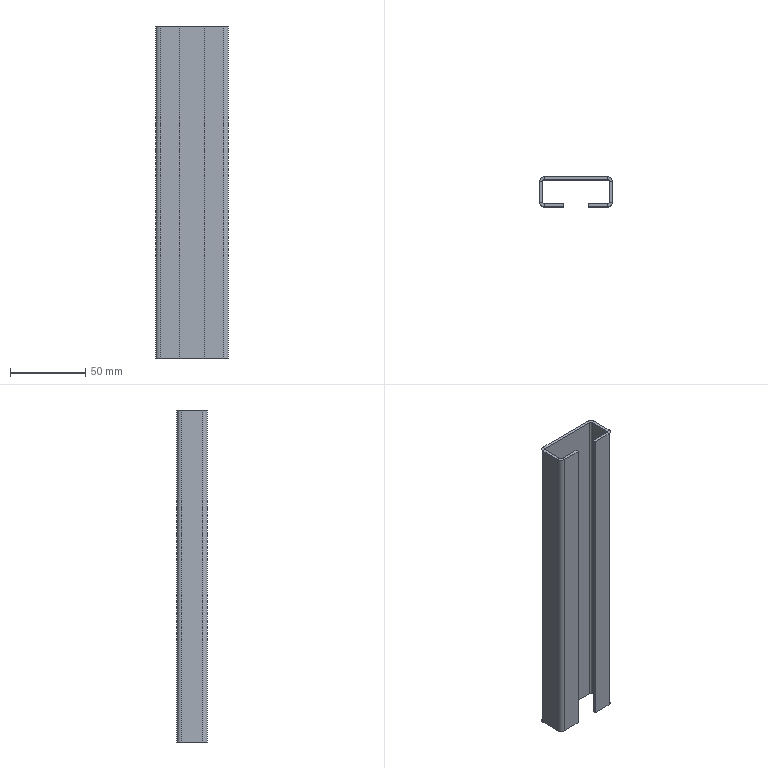Part | 1 solid | 38 faces | box 48 x 20 x 220 mm | volume 47769 mm3 | plane 30 | cylinder 8 | commonest cylinder face diameters 2 x4 6 x4
STEP:
#1=CARTESIAN_POINT('',(-24.,-17.,110.));
#2=VERTEX_POINT('',#1);
#3=CARTESIAN_POINT('',(-22.,-17.,110.));
#4=VERTEX_POINT('',#3);
#5=CARTESIAN_POINT('',(-24.,-17.,110.));
#6=DIRECTION('',(1.,0.,0.));
#7=VECTOR('',#6,1000.);
#8=LINE('',#5,#7);
#9=EDGE_CURVE('',#2,#4,#8,.T.);
#10=ORIENTED_EDGE('',*,*,#9,.F.);
#11=CARTESIAN_POINT('',(-21.,-20.,110.));
#12=VERTEX_POINT('',#11);
#13=CARTESIAN_POINT('',(-21.,-17.,110.));
#14=DIRECTION('',(0.,0.,-1.));
#15=DIRECTION('',(1.,0.,0.));
#16=AXIS2_PLACEMENT_3D('',#13,#14,#15);
#17=CIRCLE('',#16,3.);
#18=EDGE_CURVE('',#12,#2,#17,.T.);
#19=ORIENTED_EDGE('',*,*,#18,.F.);
#20=CARTESIAN_POINT('',(-21.,-18.,110.));
#21=VERTEX_POINT('',#20);
#22=CARTESIAN_POINT('',(-21.,-18.,110.));
#23=DIRECTION('',(0.,-1.,0.));
#24=VECTOR('',#23,1000.);
#25=LINE('',#22,#24);
#26=EDGE_CURVE('',#21,#12,#25,.T.);
#27=ORIENTED_EDGE('',*,*,#26,.F.);
#28=CARTESIAN_POINT('',(-21.,-17.,110.));
#29=DIRECTION('',(0.,0.,-1.));
#30=DIRECTION('',(1.,0.,0.));
#31=AXIS2_PLACEMENT_3D('',#28,#29,#30);
#32=CIRCLE('',#31,1.);
#33=EDGE_CURVE('',#21,#4,#32,.T.);
#34=ORIENTED_EDGE('',*,*,#33,.T.);
#35=EDGE_LOOP('',(#10,#19,#27,#34));
#36=FACE_OUTER_BOUND('',#35,.T.);
#37=CARTESIAN_POINT('',(-24.,-17.,110.));
#38=DIRECTION('',(0.,0.,1.));
#39=DIRECTION('',(1.,0.,0.));
#40=AXIS2_PLACEMENT_3D('',#37,#38,#39);
#41=PLANE('',#40);
#42=ADVANCED_FACE('',(#36),#41,.T.);
#43=CARTESIAN_POINT('',(-24.,-3.,110.));
#44=VERTEX_POINT('',#43);
#45=CARTESIAN_POINT('',(-24.,-20.,110.));
#46=DIRECTION('',(0.,1.,0.));
#47=VECTOR('',#46,1000.);
#48=LINE('',#45,#47);
#49=EDGE_CURVE('',#2,#44,#48,.T.);
#50=ORIENTED_EDGE('',*,*,#49,.F.);
#51=ORIENTED_EDGE('',*,*,#9,.T.);
#52=CARTESIAN_POINT('',(-22.,-3.,110.));
#53=VERTEX_POINT('',#52);
#54=CARTESIAN_POINT('',(-22.,-20.,110.));
#55=DIRECTION('',(0.,1.,0.));
#56=VECTOR('',#55,1000.);
#57=LINE('',#54,#56);
#58=EDGE_CURVE('',#4,#53,#57,.T.);
#59=ORIENTED_EDGE('',*,*,#58,.T.);
#60=CARTESIAN_POINT('',(-22.,-3.,110.));
#61=DIRECTION('',(-1.,0.,0.));
#62=VECTOR('',#61,1000.);
#63=LINE('',#60,#62);
#64=EDGE_CURVE('',#53,#44,#63,.T.);
#65=ORIENTED_EDGE('',*,*,#64,.T.);
#66=EDGE_LOOP('',(#50,#51,#59,#65));
#67=FACE_OUTER_BOUND('',#66,.T.);
#68=CARTESIAN_POINT('',(-21.,-18.,110.));
#69=DIRECTION('',(0.,0.,1.));
#70=DIRECTION('',(1.,0.,0.));
#71=AXIS2_PLACEMENT_3D('',#68,#69,#70);
#72=PLANE('',#71);
#73=ADVANCED_FACE('',(#67),#72,.T.);
#74=CARTESIAN_POINT('',(-21.,-20.,-110.));
#75=VERTEX_POINT('',#74);
#76=CARTESIAN_POINT('',(-21.,-18.,-110.));
#77=VERTEX_POINT('',#76);
#78=CARTESIAN_POINT('',(-21.,-20.,-110.));
#79=DIRECTION('',(0.,1.,0.));
#80=VECTOR('',#79,1000.);
#81=LINE('',#78,#80);
#82=EDGE_CURVE('',#75,#77,#81,.T.);
#83=ORIENTED_EDGE('',*,*,#82,.F.);
#84=CARTESIAN_POINT('',(-24.,-17.,-110.));
#85=VERTEX_POINT('',#84);
#86=CARTESIAN_POINT('',(-21.,-17.,-110.));
#87=DIRECTION('',(0.,0.,-1.));
#88=DIRECTION('',(1.,0.,0.));
#89=AXIS2_PLACEMENT_3D('',#86,#87,#88);
#90=CIRCLE('',#89,3.);
#91=EDGE_CURVE('',#75,#85,#90,.T.);
#92=ORIENTED_EDGE('',*,*,#91,.T.);
#93=CARTESIAN_POINT('',(-22.,-17.,-110.));
#94=VERTEX_POINT('',#93);
#95=CARTESIAN_POINT('',(-22.,-17.,-110.));
#96=DIRECTION('',(-1.,0.,0.));
#97=VECTOR('',#96,1000.);
#98=LINE('',#95,#97);
#99=EDGE_CURVE('',#94,#85,#98,.T.);
#100=ORIENTED_EDGE('',*,*,#99,.F.);
#101=CARTESIAN_POINT('',(-21.,-17.,-110.));
#102=DIRECTION('',(0.,0.,-1.));
#103=DIRECTION('',(1.,0.,0.));
#104=AXIS2_PLACEMENT_3D('',#101,#102,#103);
#105=CIRCLE('',#104,1.);
#106=EDGE_CURVE('',#77,#94,#105,.T.);
#107=ORIENTED_EDGE('',*,*,#106,.F.);
#108=EDGE_LOOP('',(#83,#92,#100,#107));
#109=FACE_OUTER_BOUND('',#108,.T.);
#110=CARTESIAN_POINT('',(-21.,-20.,-110.));
#111=DIRECTION('',(0.,0.,-1.));
#112=DIRECTION('',(-1.,0.,0.));
#113=AXIS2_PLACEMENT_3D('',#110,#111,#112);
#114=PLANE('',#113);
#115=ADVANCED_FACE('',(#109),#114,.T.);
#116=CARTESIAN_POINT('',(-8.,-20.,-110.));
#117=VERTEX_POINT('',#116);
#118=CARTESIAN_POINT('',(-8.,-20.,-110.));
#119=DIRECTION('',(-1.,0.,0.));
#120=VECTOR('',#119,1000.);
#121=LINE('',#118,#120);
#122=EDGE_CURVE('',#117,#75,#121,.T.);
#123=ORIENTED_EDGE('',*,*,#122,.T.);
#124=ORIENTED_EDGE('',*,*,#82,.T.);
#125=CARTESIAN_POINT('',(-8.,-18.,-110.));
#126=VERTEX_POINT('',#125);
#127=CARTESIAN_POINT('',(-8.,-18.,-110.));
#128=DIRECTION('',(-1.,0.,0.));
#129=VECTOR('',#128,1000.);
#130=LINE('',#127,#129);
#131=EDGE_CURVE('',#126,#77,#130,.T.);
#132=ORIENTED_EDGE('',*,*,#131,.F.);
#133=CARTESIAN_POINT('',(-8.,-18.,-110.));
#134=DIRECTION('',(0.,-1.,0.));
#135=VECTOR('',#134,1000.);
#136=LINE('',#133,#135);
#137=EDGE_CURVE('',#126,#117,#136,.T.);
#138=ORIENTED_EDGE('',*,*,#137,.T.);
#139=EDGE_LOOP('',(#123,#124,#132,#138));
#140=FACE_OUTER_BOUND('',#139,.T.);
#141=CARTESIAN_POINT('',(-22.,-17.,-110.));
#142=DIRECTION('',(0.,0.,-1.));
#143=DIRECTION('',(-1.,0.,0.));
#144=AXIS2_PLACEMENT_3D('',#141,#142,#143);
#145=PLANE('',#144);
#146=ADVANCED_FACE('',(#140),#145,.T.);
#147=CARTESIAN_POINT('',(-21.,0.,110.));
#148=VERTEX_POINT('',#147);
#149=CARTESIAN_POINT('',(-21.,-2.,110.));
#150=VERTEX_POINT('',#149);
#151=CARTESIAN_POINT('',(-21.,0.,110.));
#152=DIRECTION('',(0.,-1.,0.));
#153=VECTOR('',#152,1000.);
#154=LINE('',#151,#153);
#155=EDGE_CURVE('',#148,#150,#154,.T.);
#156=ORIENTED_EDGE('',*,*,#155,.F.);
#157=CARTESIAN_POINT('',(-21.,-3.,110.));
#158=DIRECTION('',(0.,0.,-1.));
#159=DIRECTION('',(1.,0.,0.));
#160=AXIS2_PLACEMENT_3D('',#157,#158,#159);
#161=CIRCLE('',#160,3.);
#162=EDGE_CURVE('',#44,#148,#161,.T.);
#163=ORIENTED_EDGE('',*,*,#162,.F.);
#164=ORIENTED_EDGE('',*,*,#64,.F.);
#165=CARTESIAN_POINT('',(-21.,-3.,110.));
#166=DIRECTION('',(0.,0.,-1.));
#167=DIRECTION('',(1.,0.,0.));
#168=AXIS2_PLACEMENT_3D('',#165,#166,#167);
#169=CIRCLE('',#168,1.);
#170=EDGE_CURVE('',#53,#150,#169,.T.);
#171=ORIENTED_EDGE('',*,*,#170,.T.);
#172=EDGE_LOOP('',(#156,#163,#164,#171));
#173=FACE_OUTER_BOUND('',#172,.T.);
#174=CARTESIAN_POINT('',(-21.,0.,110.));
#175=DIRECTION('',(0.,0.,1.));
#176=DIRECTION('',(1.,0.,0.));
#177=AXIS2_PLACEMENT_3D('',#174,#175,#176);
#178=PLANE('',#177);
#179=ADVANCED_FACE('',(#173),#178,.T.);
#180=CARTESIAN_POINT('',(21.,0.,110.));
#181=VERTEX_POINT('',#180);
#182=CARTESIAN_POINT('',(-24.,0.,110.));
#183=DIRECTION('',(1.,0.,0.));
#184=VECTOR('',#183,1000.);
#185=LINE('',#182,#184);
#186=EDGE_CURVE('',#148,#181,#185,.T.);
#187=ORIENTED_EDGE('',*,*,#186,.F.);
#188=ORIENTED_EDGE('',*,*,#155,.T.);
#189=CARTESIAN_POINT('',(21.,-2.,110.));
#190=VERTEX_POINT('',#189);
#191=CARTESIAN_POINT('',(-24.,-2.,110.));
#192=DIRECTION('',(1.,0.,0.));
#193=VECTOR('',#192,1000.);
#194=LINE('',#191,#193);
#195=EDGE_CURVE('',#150,#190,#194,.T.);
#196=ORIENTED_EDGE('',*,*,#195,.T.);
#197=CARTESIAN_POINT('',(21.,-2.,110.));
#198=DIRECTION('',(0.,1.,0.));
#199=VECTOR('',#198,1000.);
#200=LINE('',#197,#199);
#201=EDGE_CURVE('',#190,#181,#200,.T.);
#202=ORIENTED_EDGE('',*,*,#201,.T.);
#203=EDGE_LOOP('',(#187,#188,#196,#202));
#204=FACE_OUTER_BOUND('',#203,.T.);
#205=CARTESIAN_POINT('',(-22.,-3.,110.));
#206=DIRECTION('',(0.,0.,1.));
#207=DIRECTION('',(1.,0.,0.));
#208=AXIS2_PLACEMENT_3D('',#205,#206,#207);
#209=PLANE('',#208);
#210=ADVANCED_FACE('',(#204),#209,.T.);
#211=CARTESIAN_POINT('',(-24.,-3.,-110.));
#212=VERTEX_POINT('',#211);
#213=CARTESIAN_POINT('',(-22.,-3.,-110.));
#214=VERTEX_POINT('',#213);
#215=CARTESIAN_POINT('',(-24.,-3.,-110.));
#216=DIRECTION('',(1.,0.,0.));
#217=VECTOR('',#216,1000.);
#218=LINE('',#215,#217);
#219=EDGE_CURVE('',#212,#214,#218,.T.);
#220=ORIENTED_EDGE('',*,*,#219,.F.);
#221=CARTESIAN_POINT('',(-21.,0.,-110.));
#222=VERTEX_POINT('',#221);
#223=CARTESIAN_POINT('',(-21.,-3.,-110.));
#224=DIRECTION('',(0.,0.,-1.));
#225=DIRECTION('',(1.,0.,0.));
#226=AXIS2_PLACEMENT_3D('',#223,#224,#225);
#227=CIRCLE('',#226,3.);
#228=EDGE_CURVE('',#212,#222,#227,.T.);
#229=ORIENTED_EDGE('',*,*,#228,.T.);
#230=CARTESIAN_POINT('',(-21.,-2.,-110.));
#231=VERTEX_POINT('',#230);
#232=CARTESIAN_POINT('',(-21.,-2.,-110.));
#233=DIRECTION('',(0.,1.,0.));
#234=VECTOR('',#233,1000.);
#235=LINE('',#232,#234);
#236=EDGE_CURVE('',#231,#222,#235,.T.);
#237=ORIENTED_EDGE('',*,*,#236,.F.);
#238=CARTESIAN_POINT('',(-21.,-3.,-110.));
#239=DIRECTION('',(0.,0.,-1.));
#240=DIRECTION('',(1.,0.,0.));
#241=AXIS2_PLACEMENT_3D('',#238,#239,#240);
#242=CIRCLE('',#241,1.);
#243=EDGE_CURVE('',#214,#231,#242,.T.);
#244=ORIENTED_EDGE('',*,*,#243,.F.);
#245=EDGE_LOOP('',(#220,#229,#237,#244));
#246=FACE_OUTER_BOUND('',#245,.T.);
#247=CARTESIAN_POINT('',(-24.,-3.,-110.));
#248=DIRECTION('',(0.,0.,-1.));
#249=DIRECTION('',(-1.,0.,0.));
#250=AXIS2_PLACEMENT_3D('',#247,#248,#249);
#251=PLANE('',#250);
#252=ADVANCED_FACE('',(#246),#251,.T.);
#253=CARTESIAN_POINT('',(-24.,-20.,-110.));
#254=DIRECTION('',(0.,1.,0.));
#255=VECTOR('',#254,1000.);
#256=LINE('',#253,#255);
#257=EDGE_CURVE('',#85,#212,#256,.T.);
#258=ORIENTED_EDGE('',*,*,#257,.T.);
#259=ORIENTED_EDGE('',*,*,#219,.T.);
#260=CARTESIAN_POINT('',(-22.,-20.,-110.));
#261=DIRECTION('',(0.,1.,0.));
#262=VECTOR('',#261,1000.);
#263=LINE('',#260,#262);
#264=EDGE_CURVE('',#94,#214,#263,.T.);
#265=ORIENTED_EDGE('',*,*,#264,.F.);
#266=ORIENTED_EDGE('',*,*,#99,.T.);
#267=EDGE_LOOP('',(#258,#259,#265,#266));
#268=FACE_OUTER_BOUND('',#267,.T.);
#269=CARTESIAN_POINT('',(-21.,-2.,-110.));
#270=DIRECTION('',(0.,0.,-1.));
#271=DIRECTION('',(-1.,0.,0.));
#272=AXIS2_PLACEMENT_3D('',#269,#270,#271);
#273=PLANE('',#272);
#274=ADVANCED_FACE('',(#268),#273,.T.);
#275=CARTESIAN_POINT('',(24.,-3.,110.));
#276=VERTEX_POINT('',#275);
#277=CARTESIAN_POINT('',(22.,-3.,110.));
#278=VERTEX_POINT('',#277);
#279=CARTESIAN_POINT('',(24.,-3.,110.));
#280=DIRECTION('',(-1.,0.,0.));
#281=VECTOR('',#280,1000.);
#282=LINE('',#279,#281);
#283=EDGE_CURVE('',#276,#278,#282,.T.);
#284=ORIENTED_EDGE('',*,*,#283,.F.);
#285=CARTESIAN_POINT('',(21.,-3.,110.));
#286=DIRECTION('',(0.,0.,-1.));
#287=DIRECTION('',(1.,0.,0.));
#288=AXIS2_PLACEMENT_3D('',#285,#286,#287);
#289=CIRCLE('',#288,3.);
#290=EDGE_CURVE('',#181,#276,#289,.T.);
#291=ORIENTED_EDGE('',*,*,#290,.F.);
#292=ORIENTED_EDGE('',*,*,#201,.F.);
#293=CARTESIAN_POINT('',(21.,-3.,110.));
#294=DIRECTION('',(0.,0.,-1.));
#295=DIRECTION('',(1.,0.,0.));
#296=AXIS2_PLACEMENT_3D('',#293,#294,#295);
#297=CIRCLE('',#296,1.);
#298=EDGE_CURVE('',#190,#278,#297,.T.);
#299=ORIENTED_EDGE('',*,*,#298,.T.);
#300=EDGE_LOOP('',(#284,#291,#292,#299));
#301=FACE_OUTER_BOUND('',#300,.T.);
#302=CARTESIAN_POINT('',(24.,-3.,110.));
#303=DIRECTION('',(0.,0.,1.));
#304=DIRECTION('',(1.,0.,0.));
#305=AXIS2_PLACEMENT_3D('',#302,#303,#304);
#306=PLANE('',#305);
#307=ADVANCED_FACE('',(#301),#306,.T.);
#308=CARTESIAN_POINT('',(24.,-17.,110.));
#309=VERTEX_POINT('',#308);
#310=CARTESIAN_POINT('',(24.,0.,110.));
#311=DIRECTION('',(0.,-1.,0.));
#312=VECTOR('',#311,1000.);
#313=LINE('',#310,#312);
#314=EDGE_CURVE('',#276,#309,#313,.T.);
#315=ORIENTED_EDGE('',*,*,#314,.F.);
#316=ORIENTED_EDGE('',*,*,#283,.T.);
#317=CARTESIAN_POINT('',(22.,-17.,110.));
#318=VERTEX_POINT('',#317);
#319=CARTESIAN_POINT('',(22.,0.,110.));
#320=DIRECTION('',(0.,-1.,0.));
#321=VECTOR('',#320,1000.);
#322=LINE('',#319,#321);
#323=EDGE_CURVE('',#278,#318,#322,.T.);
#324=ORIENTED_EDGE('',*,*,#323,.T.);
#325=CARTESIAN_POINT('',(22.,-17.,110.));
#326=DIRECTION('',(1.,0.,0.));
#327=VECTOR('',#326,1000.);
#328=LINE('',#325,#327);
#329=EDGE_CURVE('',#318,#309,#328,.T.);
#330=ORIENTED_EDGE('',*,*,#329,.T.);
#331=EDGE_LOOP('',(#315,#316,#324,#330));
#332=FACE_OUTER_BOUND('',#331,.T.);
#333=CARTESIAN_POINT('',(21.,-2.,110.));
#334=DIRECTION('',(0.,0.,1.));
#335=DIRECTION('',(1.,0.,0.));
#336=AXIS2_PLACEMENT_3D('',#333,#334,#335);
#337=PLANE('',#336);
#338=ADVANCED_FACE('',(#332),#337,.T.);
#339=CARTESIAN_POINT('',(21.,0.,-110.));
#340=VERTEX_POINT('',#339);
#341=CARTESIAN_POINT('',(21.,-2.,-110.));
#342=VERTEX_POINT('',#341);
#343=CARTESIAN_POINT('',(21.,0.,-110.));
#344=DIRECTION('',(0.,-1.,0.));
#345=VECTOR('',#344,1000.);
#346=LINE('',#343,#345);
#347=EDGE_CURVE('',#340,#342,#346,.T.);
#348=ORIENTED_EDGE('',*,*,#347,.F.);
#349=CARTESIAN_POINT('',(24.,-3.,-110.));
#350=VERTEX_POINT('',#349);
#351=CARTESIAN_POINT('',(21.,-3.,-110.));
#352=DIRECTION('',(0.,0.,-1.));
#353=DIRECTION('',(1.,0.,0.));
#354=AXIS2_PLACEMENT_3D('',#351,#352,#353);
#355=CIRCLE('',#354,3.);
#356=EDGE_CURVE('',#340,#350,#355,.T.);
#357=ORIENTED_EDGE('',*,*,#356,.T.);
#358=CARTESIAN_POINT('',(22.,-3.,-110.));
#359=VERTEX_POINT('',#358);
#360=CARTESIAN_POINT('',(22.,-3.,-110.));
#361=DIRECTION('',(1.,0.,0.));
#362=VECTOR('',#361,1000.);
#363=LINE('',#360,#362);
#364=EDGE_CURVE('',#359,#350,#363,.T.);
#365=ORIENTED_EDGE('',*,*,#364,.F.);
#366=CARTESIAN_POINT('',(21.,-3.,-110.));
#367=DIRECTION('',(0.,0.,-1.));
#368=DIRECTION('',(1.,0.,0.));
#369=AXIS2_PLACEMENT_3D('',#366,#367,#368);
#370=CIRCLE('',#369,1.);
#371=EDGE_CURVE('',#342,#359,#370,.T.);
#372=ORIENTED_EDGE('',*,*,#371,.F.);
#373=EDGE_LOOP('',(#348,#357,#365,#372));
#374=FACE_OUTER_BOUND('',#373,.T.);
#375=CARTESIAN_POINT('',(21.,0.,-110.));
#376=DIRECTION('',(0.,0.,-1.));
#377=DIRECTION('',(-1.,0.,0.));
#378=AXIS2_PLACEMENT_3D('',#375,#376,#377);
#379=PLANE('',#378);
#380=ADVANCED_FACE('',(#374),#379,.T.);
#381=CARTESIAN_POINT('',(-24.,0.,-110.));
#382=DIRECTION('',(1.,0.,0.));
#383=VECTOR('',#382,1000.);
#384=LINE('',#381,#383);
#385=EDGE_CURVE('',#222,#340,#384,.T.);
#386=ORIENTED_EDGE('',*,*,#385,.T.);
#387=ORIENTED_EDGE('',*,*,#347,.T.);
#388=CARTESIAN_POINT('',(-24.,-2.,-110.));
#389=DIRECTION('',(1.,0.,0.));
#390=VECTOR('',#389,1000.);
#391=LINE('',#388,#390);
#392=EDGE_CURVE('',#231,#342,#391,.T.);
#393=ORIENTED_EDGE('',*,*,#392,.F.);
#394=ORIENTED_EDGE('',*,*,#236,.T.);
#395=EDGE_LOOP('',(#386,#387,#393,#394));
#396=FACE_OUTER_BOUND('',#395,.T.);
#397=CARTESIAN_POINT('',(22.,-3.,-110.));
#398=DIRECTION('',(0.,0.,-1.));
#399=DIRECTION('',(-1.,0.,0.));
#400=AXIS2_PLACEMENT_3D('',#397,#398,#399);
#401=PLANE('',#400);
#402=ADVANCED_FACE('',(#396),#401,.T.);
#403=CARTESIAN_POINT('',(21.,-20.,110.));
#404=VERTEX_POINT('',#403);
#405=CARTESIAN_POINT('',(21.,-18.,110.));
#406=VERTEX_POINT('',#405);
#407=CARTESIAN_POINT('',(21.,-20.,110.));
#408=DIRECTION('',(0.,1.,0.));
#409=VECTOR('',#408,1000.);
#410=LINE('',#407,#409);
#411=EDGE_CURVE('',#404,#406,#410,.T.);
#412=ORIENTED_EDGE('',*,*,#411,.F.);
#413=CARTESIAN_POINT('',(21.,-17.,110.));
#414=DIRECTION('',(0.,0.,-1.));
#415=DIRECTION('',(1.,0.,0.));
#416=AXIS2_PLACEMENT_3D('',#413,#414,#415);
#417=CIRCLE('',#416,3.);
#418=EDGE_CURVE('',#309,#404,#417,.T.);
#419=ORIENTED_EDGE('',*,*,#418,.F.);
#420=ORIENTED_EDGE('',*,*,#329,.F.);
#421=CARTESIAN_POINT('',(21.,-17.,110.));
#422=DIRECTION('',(0.,0.,-1.));
#423=DIRECTION('',(1.,0.,0.));
#424=AXIS2_PLACEMENT_3D('',#421,#422,#423);
#425=CIRCLE('',#424,1.);
#426=EDGE_CURVE('',#318,#406,#425,.T.);
#427=ORIENTED_EDGE('',*,*,#426,.T.);
#428=EDGE_LOOP('',(#412,#419,#420,#427));
#429=FACE_OUTER_BOUND('',#428,.T.);
#430=CARTESIAN_POINT('',(21.,-20.,110.));
#431=DIRECTION('',(0.,0.,1.));
#432=DIRECTION('',(1.,0.,0.));
#433=AXIS2_PLACEMENT_3D('',#430,#431,#432);
#434=PLANE('',#433);
#435=ADVANCED_FACE('',(#429),#434,.T.);
#436=CARTESIAN_POINT('',(8.,-20.,110.));
#437=VERTEX_POINT('',#436);
#438=CARTESIAN_POINT('',(24.,-20.,110.));
#439=DIRECTION('',(-1.,0.,0.));
#440=VECTOR('',#439,1000.);
#441=LINE('',#438,#440);
#442=EDGE_CURVE('',#404,#437,#441,.T.);
#443=ORIENTED_EDGE('',*,*,#442,.F.);
#444=ORIENTED_EDGE('',*,*,#411,.T.);
#445=CARTESIAN_POINT('',(8.,-18.,110.));
#446=VERTEX_POINT('',#445);
#447=CARTESIAN_POINT('',(24.,-18.,110.));
#448=DIRECTION('',(-1.,0.,0.));
#449=VECTOR('',#448,1000.);
#450=LINE('',#447,#449);
#451=EDGE_CURVE('',#406,#446,#450,.T.);
#452=ORIENTED_EDGE('',*,*,#451,.T.);
#453=CARTESIAN_POINT('',(8.,-20.,110.));
#454=DIRECTION('',(0.,1.,0.));
#455=VECTOR('',#454,1000.);
#456=LINE('',#453,#455);
#457=EDGE_CURVE('',#437,#446,#456,.T.);
#458=ORIENTED_EDGE('',*,*,#457,.F.);
#459=EDGE_LOOP('',(#443,#444,#452,#458));
#460=FACE_OUTER_BOUND('',#459,.T.);
#461=CARTESIAN_POINT('',(22.,-17.,110.));
#462=DIRECTION('',(0.,0.,1.));
#463=DIRECTION('',(1.,0.,0.));
#464=AXIS2_PLACEMENT_3D('',#461,#462,#463);
#465=PLANE('',#464);
#466=ADVANCED_FACE('',(#460),#465,.T.);
#467=CARTESIAN_POINT('',(24.,-17.,-110.));
#468=VERTEX_POINT('',#467);
#469=CARTESIAN_POINT('',(22.,-17.,-110.));
#470=VERTEX_POINT('',#469);
#471=CARTESIAN_POINT('',(24.,-17.,-110.));
#472=DIRECTION('',(-1.,0.,0.));
#473=VECTOR('',#472,1000.);
#474=LINE('',#471,#473);
#475=EDGE_CURVE('',#468,#470,#474,.T.);
#476=ORIENTED_EDGE('',*,*,#475,.F.);
#477=CARTESIAN_POINT('',(21.,-20.,-110.));
#478=VERTEX_POINT('',#477);
#479=CARTESIAN_POINT('',(21.,-17.,-110.));
#480=DIRECTION('',(0.,0.,-1.));
#481=DIRECTION('',(1.,0.,0.));
#482=AXIS2_PLACEMENT_3D('',#479,#480,#481);
#483=CIRCLE('',#482,3.);
#484=EDGE_CURVE('',#468,#478,#483,.T.);
#485=ORIENTED_EDGE('',*,*,#484,.T.);
#486=CARTESIAN_POINT('',(21.,-18.,-110.));
#487=VERTEX_POINT('',#486);
#488=CARTESIAN_POINT('',(21.,-18.,-110.));
#489=DIRECTION('',(0.,-1.,0.));
#490=VECTOR('',#489,1000.);
#491=LINE('',#488,#490);
#492=EDGE_CURVE('',#487,#478,#491,.T.);
#493=ORIENTED_EDGE('',*,*,#492,.F.);
#494=CARTESIAN_POINT('',(21.,-17.,-110.));
#495=DIRECTION('',(0.,0.,-1.));
#496=DIRECTION('',(1.,0.,0.));
#497=AXIS2_PLACEMENT_3D('',#494,#495,#496);
#498=CIRCLE('',#497,1.);
#499=EDGE_CURVE('',#470,#487,#498,.T.);
#500=ORIENTED_EDGE('',*,*,#499,.F.);
#501=EDGE_LOOP('',(#476,#485,#493,#500));
#502=FACE_OUTER_BOUND('',#501,.T.);
#503=CARTESIAN_POINT('',(24.,-17.,-110.));
#504=DIRECTION('',(0.,0.,-1.));
#505=DIRECTION('',(-1.,0.,0.));
#506=AXIS2_PLACEMENT_3D('',#503,#504,#505);
#507=PLANE('',#506);
#508=ADVANCED_FACE('',(#502),#507,.T.);
#509=CARTESIAN_POINT('',(24.,0.,-110.));
#510=DIRECTION('',(0.,-1.,0.));
#511=VECTOR('',#510,1000.);
#512=LINE('',#509,#511);
#513=EDGE_CURVE('',#350,#468,#512,.T.);
#514=ORIENTED_EDGE('',*,*,#513,.T.);
#515=ORIENTED_EDGE('',*,*,#475,.T.);
#516=CARTESIAN_POINT('',(22.,0.,-110.));
#517=DIRECTION('',(0.,-1.,0.));
#518=VECTOR('',#517,1000.);
#519=LINE('',#516,#518);
#520=EDGE_CURVE('',#359,#470,#519,.T.);
#521=ORIENTED_EDGE('',*,*,#520,.F.);
#522=ORIENTED_EDGE('',*,*,#364,.T.);
#523=EDGE_LOOP('',(#514,#515,#521,#522));
#524=FACE_OUTER_BOUND('',#523,.T.);
#525=CARTESIAN_POINT('',(21.,-18.,-110.));
#526=DIRECTION('',(0.,0.,-1.));
#527=DIRECTION('',(-1.,0.,0.));
#528=AXIS2_PLACEMENT_3D('',#525,#526,#527);
#529=PLANE('',#528);
#530=ADVANCED_FACE('',(#524),#529,.T.);
#531=CARTESIAN_POINT('',(8.,-18.,-110.));
#532=VERTEX_POINT('',#531);
#533=CARTESIAN_POINT('',(24.,-18.,-110.));
#534=DIRECTION('',(-1.,0.,0.));
#535=VECTOR('',#534,1000.);
#536=LINE('',#533,#535);
#537=EDGE_CURVE('',#487,#532,#536,.T.);
#538=ORIENTED_EDGE('',*,*,#537,.T.);
#539=CARTESIAN_POINT('',(8.,-18.,110.));
#540=DIRECTION('',(0.,0.,-1.));
#541=VECTOR('',#540,1000.);
#542=LINE('',#539,#541);
#543=EDGE_CURVE('',#446,#532,#542,.T.);
#544=ORIENTED_EDGE('',*,*,#543,.F.);
#545=ORIENTED_EDGE('',*,*,#451,.F.);
#546=CARTESIAN_POINT('',(21.,-18.,110.));
#547=DIRECTION('',(0.,0.,-1.));
#548=VECTOR('',#547,1000.);
#549=LINE('',#546,#548);
#550=EDGE_CURVE('',#406,#487,#549,.T.);
#551=ORIENTED_EDGE('',*,*,#550,.T.);
#552=EDGE_LOOP('',(#538,#544,#545,#551));
#553=FACE_OUTER_BOUND('',#552,.T.);
#554=CARTESIAN_POINT('',(24.,-18.,110.));
#555=DIRECTION('',(0.,-1.,0.));
#556=DIRECTION('',(1.,0.,0.));
#557=AXIS2_PLACEMENT_3D('',#554,#555,#556);
#558=PLANE('',#557);
#559=ADVANCED_FACE('',(#553),#558,.F.);
#560=CARTESIAN_POINT('',(8.,-20.,-110.));
#561=VERTEX_POINT('',#560);
#562=CARTESIAN_POINT('',(8.,-20.,-110.));
#563=DIRECTION('',(0.,1.,0.));
#564=VECTOR('',#563,1000.);
#565=LINE('',#562,#564);
#566=EDGE_CURVE('',#561,#532,#565,.T.);
#567=ORIENTED_EDGE('',*,*,#566,.F.);
#568=CARTESIAN_POINT('',(8.,-20.,110.));
#569=DIRECTION('',(0.,0.,-1.));
#570=VECTOR('',#569,1000.);
#571=LINE('',#568,#570);
#572=EDGE_CURVE('',#437,#561,#571,.T.);
#573=ORIENTED_EDGE('',*,*,#572,.F.);
#574=ORIENTED_EDGE('',*,*,#457,.T.);
#575=ORIENTED_EDGE('',*,*,#543,.T.);
#576=EDGE_LOOP('',(#567,#573,#574,#575));
#577=FACE_OUTER_BOUND('',#576,.T.);
#578=CARTESIAN_POINT('',(8.,-20.,110.));
#579=DIRECTION('',(-1.,0.,0.));
#580=DIRECTION('',(0.,0.,1.));
#581=AXIS2_PLACEMENT_3D('',#578,#579,#580);
#582=PLANE('',#581);
#583=ADVANCED_FACE('',(#577),#582,.T.);
#584=CARTESIAN_POINT('',(24.,-20.,-110.));
#585=DIRECTION('',(-1.,0.,0.));
#586=VECTOR('',#585,1000.);
#587=LINE('',#584,#586);
#588=EDGE_CURVE('',#478,#561,#587,.T.);
#589=ORIENTED_EDGE('',*,*,#588,.F.);
#590=CARTESIAN_POINT('',(21.,-20.,110.));
#591=DIRECTION('',(0.,0.,-1.));
#592=VECTOR('',#591,1000.);
#593=LINE('',#590,#592);
#594=EDGE_CURVE('',#404,#478,#593,.T.);
#595=ORIENTED_EDGE('',*,*,#594,.F.);
#596=ORIENTED_EDGE('',*,*,#442,.T.);
#597=ORIENTED_EDGE('',*,*,#572,.T.);
#598=EDGE_LOOP('',(#589,#595,#596,#597));
#599=FACE_OUTER_BOUND('',#598,.T.);
#600=CARTESIAN_POINT('',(24.,-20.,110.));
#601=DIRECTION('',(0.,-1.,0.));
#602=DIRECTION('',(1.,0.,0.));
#603=AXIS2_PLACEMENT_3D('',#600,#601,#602);
#604=PLANE('',#603);
#605=ADVANCED_FACE('',(#599),#604,.T.);
#606=ORIENTED_EDGE('',*,*,#484,.F.);
#607=CARTESIAN_POINT('',(24.,-17.,110.));
#608=DIRECTION('',(0.,0.,-1.));
#609=VECTOR('',#608,1000.);
#610=LINE('',#607,#609);
#611=EDGE_CURVE('',#309,#468,#610,.T.);
#612=ORIENTED_EDGE('',*,*,#611,.F.);
#613=ORIENTED_EDGE('',*,*,#418,.T.);
#614=ORIENTED_EDGE('',*,*,#594,.T.);
#615=EDGE_LOOP('',(#606,#612,#613,#614));
#616=FACE_OUTER_BOUND('',#615,.T.);
#617=CARTESIAN_POINT('',(21.,-17.,110.));
#618=DIRECTION('',(0.,0.,-1.));
#619=DIRECTION('',(-1.,0.,0.));
#620=AXIS2_PLACEMENT_3D('',#617,#618,#619);
#621=CYLINDRICAL_SURFACE('',#620,3.);
#622=ADVANCED_FACE('',(#616),#621,.T.);
#623=ORIENTED_EDGE('',*,*,#513,.F.);
#624=CARTESIAN_POINT('',(24.,-3.,110.));
#625=DIRECTION('',(0.,0.,-1.));
#626=VECTOR('',#625,1000.);
#627=LINE('',#624,#626);
#628=EDGE_CURVE('',#276,#350,#627,.T.);
#629=ORIENTED_EDGE('',*,*,#628,.F.);
#630=ORIENTED_EDGE('',*,*,#314,.T.);
#631=ORIENTED_EDGE('',*,*,#611,.T.);
#632=EDGE_LOOP('',(#623,#629,#630,#631));
#633=FACE_OUTER_BOUND('',#632,.T.);
#634=CARTESIAN_POINT('',(24.,0.,110.));
#635=DIRECTION('',(1.,0.,0.));
#636=DIRECTION('',(0.,0.,-1.));
#637=AXIS2_PLACEMENT_3D('',#634,#635,#636);
#638=PLANE('',#637);
#639=ADVANCED_FACE('',(#633),#638,.T.);
#640=ORIENTED_EDGE('',*,*,#356,.F.);
#641=CARTESIAN_POINT('',(21.,0.,110.));
#642=DIRECTION('',(0.,0.,-1.));
#643=VECTOR('',#642,1000.);
#644=LINE('',#641,#643);
#645=EDGE_CURVE('',#181,#340,#644,.T.);
#646=ORIENTED_EDGE('',*,*,#645,.F.);
#647=ORIENTED_EDGE('',*,*,#290,.T.);
#648=ORIENTED_EDGE('',*,*,#628,.T.);
#649=EDGE_LOOP('',(#640,#646,#647,#648));
#650=FACE_OUTER_BOUND('',#649,.T.);
#651=CARTESIAN_POINT('',(21.,-3.,110.));
#652=DIRECTION('',(0.,0.,-1.));
#653=DIRECTION('',(-1.,0.,0.));
#654=AXIS2_PLACEMENT_3D('',#651,#652,#653);
#655=CYLINDRICAL_SURFACE('',#654,3.);
#656=ADVANCED_FACE('',(#650),#655,.T.);
#657=ORIENTED_EDGE('',*,*,#385,.F.);
#658=CARTESIAN_POINT('',(-21.,0.,110.));
#659=DIRECTION('',(0.,0.,-1.));
#660=VECTOR('',#659,1000.);
#661=LINE('',#658,#660);
#662=EDGE_CURVE('',#148,#222,#661,.T.);
#663=ORIENTED_EDGE('',*,*,#662,.F.);
#664=ORIENTED_EDGE('',*,*,#186,.T.);
#665=ORIENTED_EDGE('',*,*,#645,.T.);
#666=EDGE_LOOP('',(#657,#663,#664,#665));
#667=FACE_OUTER_BOUND('',#666,.T.);
#668=CARTESIAN_POINT('',(-24.,0.,110.));
#669=DIRECTION('',(0.,1.,0.));
#670=DIRECTION('',(0.,0.,1.));
#671=AXIS2_PLACEMENT_3D('',#668,#669,#670);
#672=PLANE('',#671);
#673=ADVANCED_FACE('',(#667),#672,.T.);
#674=ORIENTED_EDGE('',*,*,#228,.F.);
#675=CARTESIAN_POINT('',(-24.,-3.,110.));
#676=DIRECTION('',(0.,0.,-1.));
#677=VECTOR('',#676,1000.);
#678=LINE('',#675,#677);
#679=EDGE_CURVE('',#44,#212,#678,.T.);
#680=ORIENTED_EDGE('',*,*,#679,.F.);
#681=ORIENTED_EDGE('',*,*,#162,.T.);
#682=ORIENTED_EDGE('',*,*,#662,.T.);
#683=EDGE_LOOP('',(#674,#680,#681,#682));
#684=FACE_OUTER_BOUND('',#683,.T.);
#685=CARTESIAN_POINT('',(-21.,-3.,110.));
#686=DIRECTION('',(0.,0.,-1.));
#687=DIRECTION('',(-1.,0.,0.));
#688=AXIS2_PLACEMENT_3D('',#685,#686,#687);
#689=CYLINDRICAL_SURFACE('',#688,3.);
#690=ADVANCED_FACE('',(#684),#689,.T.);
#691=ORIENTED_EDGE('',*,*,#257,.F.);
#692=CARTESIAN_POINT('',(-24.,-17.,110.));
#693=DIRECTION('',(0.,0.,-1.));
#694=VECTOR('',#693,1000.);
#695=LINE('',#692,#694);
#696=EDGE_CURVE('',#2,#85,#695,.T.);
#697=ORIENTED_EDGE('',*,*,#696,.F.);
#698=ORIENTED_EDGE('',*,*,#49,.T.);
#699=ORIENTED_EDGE('',*,*,#679,.T.);
#700=EDGE_LOOP('',(#691,#697,#698,#699));
#701=FACE_OUTER_BOUND('',#700,.T.);
#702=CARTESIAN_POINT('',(-24.,-20.,110.));
#703=DIRECTION('',(-1.,0.,0.));
#704=DIRECTION('',(0.,0.,1.));
#705=AXIS2_PLACEMENT_3D('',#702,#703,#704);
#706=PLANE('',#705);
#707=ADVANCED_FACE('',(#701),#706,.T.);
#708=ORIENTED_EDGE('',*,*,#91,.F.);
#709=CARTESIAN_POINT('',(-21.,-20.,110.));
#710=DIRECTION('',(0.,0.,-1.));
#711=VECTOR('',#710,1000.);
#712=LINE('',#709,#711);
#713=EDGE_CURVE('',#12,#75,#712,.T.);
#714=ORIENTED_EDGE('',*,*,#713,.F.);
#715=ORIENTED_EDGE('',*,*,#18,.T.);
#716=ORIENTED_EDGE('',*,*,#696,.T.);
#717=EDGE_LOOP('',(#708,#714,#715,#716));
#718=FACE_OUTER_BOUND('',#717,.T.);
#719=CARTESIAN_POINT('',(-21.,-17.,110.));
#720=DIRECTION('',(0.,0.,-1.));
#721=DIRECTION('',(-1.,0.,0.));
#722=AXIS2_PLACEMENT_3D('',#719,#720,#721);
#723=CYLINDRICAL_SURFACE('',#722,3.);
#724=ADVANCED_FACE('',(#718),#723,.T.);
#725=ORIENTED_EDGE('',*,*,#122,.F.);
#726=CARTESIAN_POINT('',(-8.,-20.,110.));
#727=VERTEX_POINT('',#726);
#728=CARTESIAN_POINT('',(-8.,-20.,110.));
#729=DIRECTION('',(0.,0.,-1.));
#730=VECTOR('',#729,1000.);
#731=LINE('',#728,#730);
#732=EDGE_CURVE('',#727,#117,#731,.T.);
#733=ORIENTED_EDGE('',*,*,#732,.F.);
#734=CARTESIAN_POINT('',(-8.,-20.,110.));
#735=DIRECTION('',(-1.,0.,0.));
#736=VECTOR('',#735,1000.);
#737=LINE('',#734,#736);
#738=EDGE_CURVE('',#727,#12,#737,.T.);
#739=ORIENTED_EDGE('',*,*,#738,.T.);
#740=ORIENTED_EDGE('',*,*,#713,.T.);
#741=EDGE_LOOP('',(#725,#733,#739,#740));
#742=FACE_OUTER_BOUND('',#741,.T.);
#743=CARTESIAN_POINT('',(-8.,-20.,110.));
#744=DIRECTION('',(0.,-1.,0.));
#745=DIRECTION('',(1.,0.,0.));
#746=AXIS2_PLACEMENT_3D('',#743,#744,#745);
#747=PLANE('',#746);
#748=ADVANCED_FACE('',(#742),#747,.T.);
#749=ORIENTED_EDGE('',*,*,#137,.F.);
#750=CARTESIAN_POINT('',(-8.,-18.,110.));
#751=VERTEX_POINT('',#750);
#752=CARTESIAN_POINT('',(-8.,-18.,110.));
#753=DIRECTION('',(0.,0.,-1.));
#754=VECTOR('',#753,1000.);
#755=LINE('',#752,#754);
#756=EDGE_CURVE('',#751,#126,#755,.T.);
#757=ORIENTED_EDGE('',*,*,#756,.F.);
#758=CARTESIAN_POINT('',(-8.,-18.,110.));
#759=DIRECTION('',(0.,-1.,0.));
#760=VECTOR('',#759,1000.);
#761=LINE('',#758,#760);
#762=EDGE_CURVE('',#751,#727,#761,.T.);
#763=ORIENTED_EDGE('',*,*,#762,.T.);
#764=ORIENTED_EDGE('',*,*,#732,.T.);
#765=EDGE_LOOP('',(#749,#757,#763,#764));
#766=FACE_OUTER_BOUND('',#765,.T.);
#767=CARTESIAN_POINT('',(-8.,-18.,110.));
#768=DIRECTION('',(1.,0.,0.));
#769=DIRECTION('',(0.,0.,-1.));
#770=AXIS2_PLACEMENT_3D('',#767,#768,#769);
#771=PLANE('',#770);
#772=ADVANCED_FACE('',(#766),#771,.T.);
#773=ORIENTED_EDGE('',*,*,#131,.T.);
#774=CARTESIAN_POINT('',(-21.,-18.,110.));
#775=DIRECTION('',(0.,0.,-1.));
#776=VECTOR('',#775,1000.);
#777=LINE('',#774,#776);
#778=EDGE_CURVE('',#21,#77,#777,.T.);
#779=ORIENTED_EDGE('',*,*,#778,.F.);
#780=CARTESIAN_POINT('',(-8.,-18.,110.));
#781=DIRECTION('',(-1.,0.,0.));
#782=VECTOR('',#781,1000.);
#783=LINE('',#780,#782);
#784=EDGE_CURVE('',#751,#21,#783,.T.);
#785=ORIENTED_EDGE('',*,*,#784,.F.);
#786=ORIENTED_EDGE('',*,*,#756,.T.);
#787=EDGE_LOOP('',(#773,#779,#785,#786));
#788=FACE_OUTER_BOUND('',#787,.T.);
#789=CARTESIAN_POINT('',(-8.,-18.,110.));
#790=DIRECTION('',(0.,-1.,0.));
#791=DIRECTION('',(1.,0.,0.));
#792=AXIS2_PLACEMENT_3D('',#789,#790,#791);
#793=PLANE('',#792);
#794=ADVANCED_FACE('',(#788),#793,.F.);
#795=ORIENTED_EDGE('',*,*,#106,.T.);
#796=CARTESIAN_POINT('',(-22.,-17.,110.));
#797=DIRECTION('',(0.,0.,-1.));
#798=VECTOR('',#797,1000.);
#799=LINE('',#796,#798);
#800=EDGE_CURVE('',#4,#94,#799,.T.);
#801=ORIENTED_EDGE('',*,*,#800,.F.);
#802=ORIENTED_EDGE('',*,*,#33,.F.);
#803=ORIENTED_EDGE('',*,*,#778,.T.);
#804=EDGE_LOOP('',(#795,#801,#802,#803));
#805=FACE_OUTER_BOUND('',#804,.T.);
#806=CARTESIAN_POINT('',(-21.,-17.,110.));
#807=DIRECTION('',(0.,0.,-1.));
#808=DIRECTION('',(-1.,0.,0.));
#809=AXIS2_PLACEMENT_3D('',#806,#807,#808);
#810=CYLINDRICAL_SURFACE('',#809,1.);
#811=ADVANCED_FACE('',(#805),#810,.F.);
#812=ORIENTED_EDGE('',*,*,#264,.T.);
#813=CARTESIAN_POINT('',(-22.,-3.,110.));
#814=DIRECTION('',(0.,0.,-1.));
#815=VECTOR('',#814,1000.);
#816=LINE('',#813,#815);
#817=EDGE_CURVE('',#53,#214,#816,.T.);
#818=ORIENTED_EDGE('',*,*,#817,.F.);
#819=ORIENTED_EDGE('',*,*,#58,.F.);
#820=ORIENTED_EDGE('',*,*,#800,.T.);
#821=EDGE_LOOP('',(#812,#818,#819,#820));
#822=FACE_OUTER_BOUND('',#821,.T.);
#823=CARTESIAN_POINT('',(-22.,-20.,110.));
#824=DIRECTION('',(-1.,0.,0.));
#825=DIRECTION('',(0.,0.,1.));
#826=AXIS2_PLACEMENT_3D('',#823,#824,#825);
#827=PLANE('',#826);
#828=ADVANCED_FACE('',(#822),#827,.F.);
#829=ORIENTED_EDGE('',*,*,#243,.T.);
#830=CARTESIAN_POINT('',(-21.,-2.,110.));
#831=DIRECTION('',(0.,0.,-1.));
#832=VECTOR('',#831,1000.);
#833=LINE('',#830,#832);
#834=EDGE_CURVE('',#150,#231,#833,.T.);
#835=ORIENTED_EDGE('',*,*,#834,.F.);
#836=ORIENTED_EDGE('',*,*,#170,.F.);
#837=ORIENTED_EDGE('',*,*,#817,.T.);
#838=EDGE_LOOP('',(#829,#835,#836,#837));
#839=FACE_OUTER_BOUND('',#838,.T.);
#840=CARTESIAN_POINT('',(-21.,-3.,110.));
#841=DIRECTION('',(0.,0.,-1.));
#842=DIRECTION('',(-1.,0.,0.));
#843=AXIS2_PLACEMENT_3D('',#840,#841,#842);
#844=CYLINDRICAL_SURFACE('',#843,1.);
#845=ADVANCED_FACE('',(#839),#844,.F.);
#846=ORIENTED_EDGE('',*,*,#392,.T.);
#847=CARTESIAN_POINT('',(21.,-2.,110.));
#848=DIRECTION('',(0.,0.,-1.));
#849=VECTOR('',#848,1000.);
#850=LINE('',#847,#849);
#851=EDGE_CURVE('',#190,#342,#850,.T.);
#852=ORIENTED_EDGE('',*,*,#851,.F.);
#853=ORIENTED_EDGE('',*,*,#195,.F.);
#854=ORIENTED_EDGE('',*,*,#834,.T.);
#855=EDGE_LOOP('',(#846,#852,#853,#854));
#856=FACE_OUTER_BOUND('',#855,.T.);
#857=CARTESIAN_POINT('',(-24.,-2.,110.));
#858=DIRECTION('',(0.,1.,0.));
#859=DIRECTION('',(0.,0.,1.));
#860=AXIS2_PLACEMENT_3D('',#857,#858,#859);
#861=PLANE('',#860);
#862=ADVANCED_FACE('',(#856),#861,.F.);
#863=ORIENTED_EDGE('',*,*,#371,.T.);
#864=CARTESIAN_POINT('',(22.,-3.,110.));
#865=DIRECTION('',(0.,0.,-1.));
#866=VECTOR('',#865,1000.);
#867=LINE('',#864,#866);
#868=EDGE_CURVE('',#278,#359,#867,.T.);
#869=ORIENTED_EDGE('',*,*,#868,.F.);
#870=ORIENTED_EDGE('',*,*,#298,.F.);
#871=ORIENTED_EDGE('',*,*,#851,.T.);
#872=EDGE_LOOP('',(#863,#869,#870,#871));
#873=FACE_OUTER_BOUND('',#872,.T.);
#874=CARTESIAN_POINT('',(21.,-3.,110.));
#875=DIRECTION('',(0.,0.,-1.));
#876=DIRECTION('',(-1.,0.,0.));
#877=AXIS2_PLACEMENT_3D('',#874,#875,#876);
#878=CYLINDRICAL_SURFACE('',#877,1.);
#879=ADVANCED_FACE('',(#873),#878,.F.);
#880=ORIENTED_EDGE('',*,*,#520,.T.);
#881=CARTESIAN_POINT('',(22.,-17.,110.));
#882=DIRECTION('',(0.,0.,-1.));
#883=VECTOR('',#882,1000.);
#884=LINE('',#881,#883);
#885=EDGE_CURVE('',#318,#470,#884,.T.);
#886=ORIENTED_EDGE('',*,*,#885,.F.);
#887=ORIENTED_EDGE('',*,*,#323,.F.);
#888=ORIENTED_EDGE('',*,*,#868,.T.);
#889=EDGE_LOOP('',(#880,#886,#887,#888));
#890=FACE_OUTER_BOUND('',#889,.T.);
#891=CARTESIAN_POINT('',(22.,0.,110.));
#892=DIRECTION('',(1.,0.,0.));
#893=DIRECTION('',(0.,0.,-1.));
#894=AXIS2_PLACEMENT_3D('',#891,#892,#893);
#895=PLANE('',#894);
#896=ADVANCED_FACE('',(#890),#895,.F.);
#897=ORIENTED_EDGE('',*,*,#499,.T.);
#898=ORIENTED_EDGE('',*,*,#550,.F.);
#899=ORIENTED_EDGE('',*,*,#426,.F.);
#900=ORIENTED_EDGE('',*,*,#885,.T.);
#901=EDGE_LOOP('',(#897,#898,#899,#900));
#902=FACE_OUTER_BOUND('',#901,.T.);
#903=CARTESIAN_POINT('',(21.,-17.,110.));
#904=DIRECTION('',(0.,0.,-1.));
#905=DIRECTION('',(-1.,0.,0.));
#906=AXIS2_PLACEMENT_3D('',#903,#904,#905);
#907=CYLINDRICAL_SURFACE('',#906,1.);
#908=ADVANCED_FACE('',(#902),#907,.F.);
#909=ORIENTED_EDGE('',*,*,#784,.T.);
#910=ORIENTED_EDGE('',*,*,#26,.T.);
#911=ORIENTED_EDGE('',*,*,#738,.F.);
#912=ORIENTED_EDGE('',*,*,#762,.F.);
#913=EDGE_LOOP('',(#909,#910,#911,#912));
#914=FACE_OUTER_BOUND('',#913,.T.);
#915=CARTESIAN_POINT('',(21.,-17.,110.));
#916=DIRECTION('',(0.,0.,1.));
#917=DIRECTION('',(1.,0.,0.));
#918=AXIS2_PLACEMENT_3D('',#915,#916,#917);
#919=PLANE('',#918);
#920=ADVANCED_FACE('',(#914),#919,.T.);
#921=ORIENTED_EDGE('',*,*,#537,.F.);
#922=ORIENTED_EDGE('',*,*,#492,.T.);
#923=ORIENTED_EDGE('',*,*,#588,.T.);
#924=ORIENTED_EDGE('',*,*,#566,.T.);
#925=EDGE_LOOP('',(#921,#922,#923,#924));
#926=FACE_OUTER_BOUND('',#925,.T.);
#927=CARTESIAN_POINT('',(21.,-17.,-110.));
#928=DIRECTION('',(0.,0.,1.));
#929=DIRECTION('',(1.,0.,0.));
#930=AXIS2_PLACEMENT_3D('',#927,#928,#929);
#931=PLANE('',#930);
#932=ADVANCED_FACE('',(#926),#931,.F.);
#933=CLOSED_SHELL('',(#42,#73,#115,#146,#179,#210,#252,#274,#307,#338,#380,#402,#435,#466,#508,#530,#559,#583,#605,#622,#639,#656,#673,#690,#707,#724,#748,#772,#794,#811,#828,#845,#862,#879,#896,#908,#920,#932));
#934=MANIFOLD_SOLID_BREP('',#933);
#935=CARTESIAN_POINT('',(0.,0.,0.));
#936=DIRECTION('',(0.,0.,1.));
#937=DIRECTION('',(1.,0.,0.));
#938=AXIS2_PLACEMENT_3D('',#935,#936,#937);
#939=(LENGTH_UNIT()NAMED_UNIT(*)SI_UNIT(.MILLI.,.METRE.));
#940=UNCERTAINTY_MEASURE_WITH_UNIT(LENGTH_MEASURE(0.00001),#939,'','');
#941=(NAMED_UNIT(*)PLANE_ANGLE_UNIT()SI_UNIT($,.RADIAN.));
#942=(NAMED_UNIT(*)SI_UNIT($,.STERADIAN.)SOLID_ANGLE_UNIT());
#943=(GEOMETRIC_REPRESENTATION_CONTEXT(3)GLOBAL_UNCERTAINTY_ASSIGNED_CONTEXT((#940))GLOBAL_UNIT_ASSIGNED_CONTEXT((#939,#941,#942))REPRESENTATION_CONTEXT('',''));
#944=ADVANCED_BREP_SHAPE_REPRESENTATION('',(#934,#938),#943);